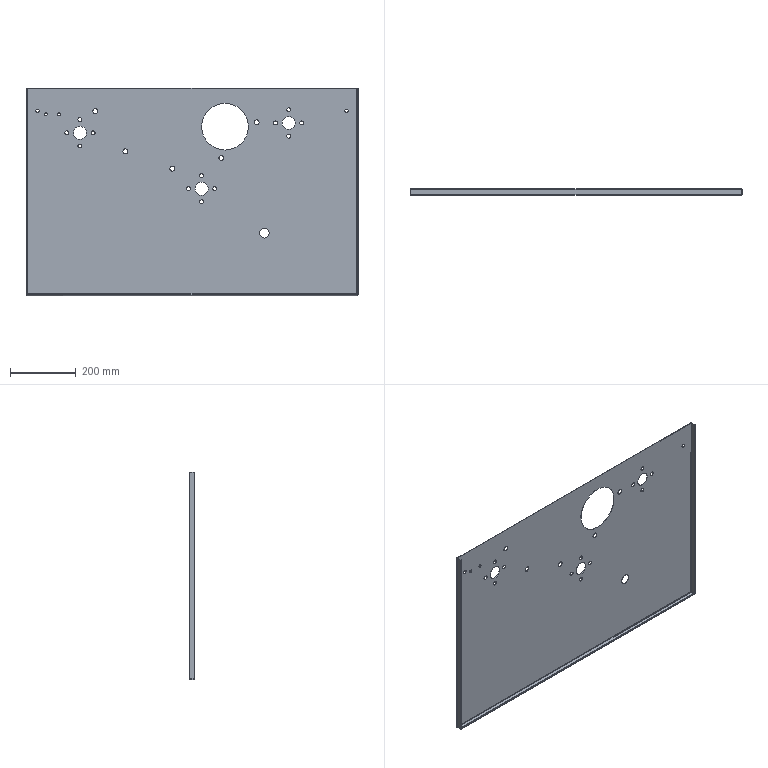Part | SolidWorks | features BaseBody 1 | 1 solid | 98 faces | box 1010 x 18 x 630 mm | volume 788896 mm3 | cylinder 64 | plane 26 | spline 8 | commonest cylinder face diameters 12 x24 15 x10 1.473 x6 3.873 x6 40 x6 8.5 x4